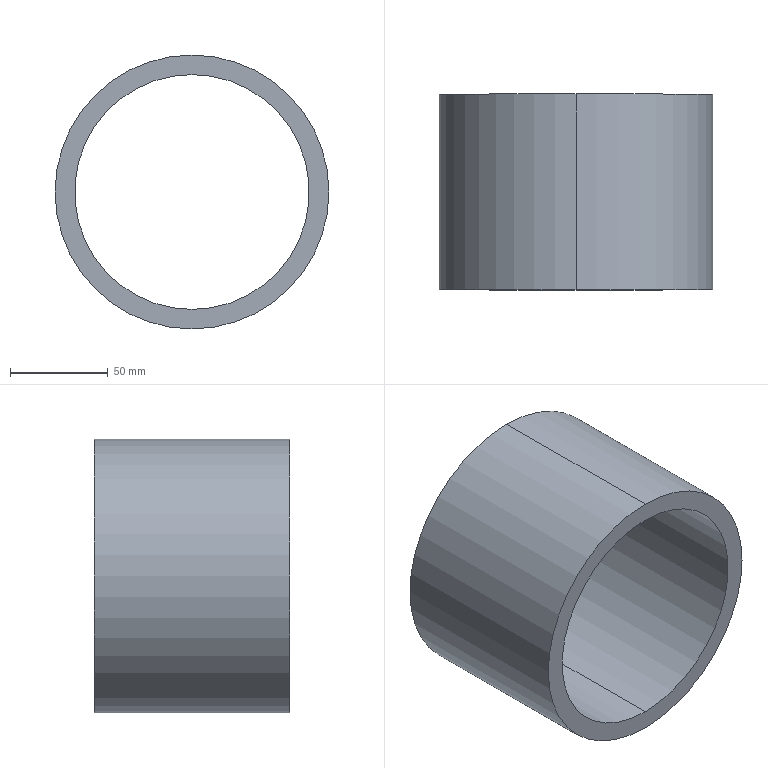Part | SolidWorks | features Extrusion 1 | 1 solid | 6 faces | box 140 x 100 x 140 mm | volume 408407 mm3 | cylinder 4 | plane 2 | commonest cylinder face diameters 120 x2 140 x2
STEP:
#1=CARTESIAN_POINT('',(0.,100.,-60.));
#2=VERTEX_POINT('',#1);
#3=CARTESIAN_POINT('',(0.,100.,60.));
#4=VERTEX_POINT('',#3);
#5=CARTESIAN_POINT('',(0.,100.,0.));
#6=DIRECTION('',(0.,1.,0.));
#7=DIRECTION('',(0.,0.,1.));
#8=AXIS2_PLACEMENT_3D('',#5,#6,#7);
#9=CIRCLE('',#8,60.);
#10=EDGE_CURVE('',#2,#4,#9,.T.);
#11=ORIENTED_EDGE('',*,*,#10,.T.);
#12=CARTESIAN_POINT('',(0.,0.,60.));
#13=VERTEX_POINT('',#12);
#14=CARTESIAN_POINT('',(0.,100.,60.));
#15=DIRECTION('',(0.,-1.,0.));
#16=VECTOR('',#15,1000.);
#17=LINE('',#14,#16);
#18=EDGE_CURVE('',#4,#13,#17,.T.);
#19=ORIENTED_EDGE('',*,*,#18,.T.);
#20=CARTESIAN_POINT('',(0.,0.,-60.));
#21=VERTEX_POINT('',#20);
#22=CARTESIAN_POINT('',(0.,0.,0.));
#23=DIRECTION('',(0.,1.,0.));
#24=DIRECTION('',(0.,0.,1.));
#25=AXIS2_PLACEMENT_3D('',#22,#23,#24);
#26=CIRCLE('',#25,60.);
#27=EDGE_CURVE('',#21,#13,#26,.T.);
#28=ORIENTED_EDGE('',*,*,#27,.F.);
#29=CARTESIAN_POINT('',(0.,100.,-60.));
#30=DIRECTION('',(0.,-1.,0.));
#31=VECTOR('',#30,1000.);
#32=LINE('',#29,#31);
#33=EDGE_CURVE('',#2,#21,#32,.T.);
#34=ORIENTED_EDGE('',*,*,#33,.F.);
#35=EDGE_LOOP('',(#11,#19,#28,#34));
#36=FACE_OUTER_BOUND('',#35,.T.);
#37=CARTESIAN_POINT('',(0.,100.,0.));
#38=DIRECTION('',(0.,-1.,0.));
#39=DIRECTION('',(0.,0.,-1.));
#40=AXIS2_PLACEMENT_3D('',#37,#38,#39);
#41=CYLINDRICAL_SURFACE('',#40,60.);
#42=ADVANCED_FACE('',(#36),#41,.F.);
#43=CARTESIAN_POINT('',(0.,100.,70.));
#44=VERTEX_POINT('',#43);
#45=CARTESIAN_POINT('',(0.,100.,-70.));
#46=VERTEX_POINT('',#45);
#47=CARTESIAN_POINT('',(0.,100.,0.));
#48=DIRECTION('',(0.,1.,0.));
#49=DIRECTION('',(0.,0.,1.));
#50=AXIS2_PLACEMENT_3D('',#47,#48,#49);
#51=CIRCLE('',#50,70.);
#52=EDGE_CURVE('',#44,#46,#51,.T.);
#53=ORIENTED_EDGE('',*,*,#52,.F.);
#54=CARTESIAN_POINT('',(0.,0.,70.));
#55=VERTEX_POINT('',#54);
#56=CARTESIAN_POINT('',(0.,100.,70.));
#57=DIRECTION('',(0.,-1.,0.));
#58=VECTOR('',#57,1000.);
#59=LINE('',#56,#58);
#60=EDGE_CURVE('',#44,#55,#59,.T.);
#61=ORIENTED_EDGE('',*,*,#60,.T.);
#62=CARTESIAN_POINT('',(0.,0.,-70.));
#63=VERTEX_POINT('',#62);
#64=CARTESIAN_POINT('',(0.,0.,0.));
#65=DIRECTION('',(0.,1.,0.));
#66=DIRECTION('',(0.,0.,1.));
#67=AXIS2_PLACEMENT_3D('',#64,#65,#66);
#68=CIRCLE('',#67,70.);
#69=EDGE_CURVE('',#55,#63,#68,.T.);
#70=ORIENTED_EDGE('',*,*,#69,.T.);
#71=CARTESIAN_POINT('',(0.,100.,-70.));
#72=DIRECTION('',(0.,-1.,0.));
#73=VECTOR('',#72,1000.);
#74=LINE('',#71,#73);
#75=EDGE_CURVE('',#46,#63,#74,.T.);
#76=ORIENTED_EDGE('',*,*,#75,.F.);
#77=EDGE_LOOP('',(#53,#61,#70,#76));
#78=FACE_OUTER_BOUND('',#77,.T.);
#79=CARTESIAN_POINT('',(0.,100.,0.));
#80=DIRECTION('',(0.,-1.,0.));
#81=DIRECTION('',(0.,0.,-1.));
#82=AXIS2_PLACEMENT_3D('',#79,#80,#81);
#83=CYLINDRICAL_SURFACE('',#82,70.);
#84=ADVANCED_FACE('',(#78),#83,.T.);
#85=CARTESIAN_POINT('',(0.,100.,0.));
#86=DIRECTION('',(0.,1.,0.));
#87=DIRECTION('',(0.,0.,1.));
#88=AXIS2_PLACEMENT_3D('',#85,#86,#87);
#89=CIRCLE('',#88,70.);
#90=EDGE_CURVE('',#46,#44,#89,.T.);
#91=ORIENTED_EDGE('',*,*,#90,.T.);
#92=ORIENTED_EDGE('',*,*,#52,.T.);
#93=EDGE_LOOP('',(#91,#92));
#94=FACE_OUTER_BOUND('',#93,.T.);
#95=ORIENTED_EDGE('',*,*,#10,.F.);
#96=CARTESIAN_POINT('',(0.,100.,0.));
#97=DIRECTION('',(0.,1.,0.));
#98=DIRECTION('',(0.,0.,1.));
#99=AXIS2_PLACEMENT_3D('',#96,#97,#98);
#100=CIRCLE('',#99,60.);
#101=EDGE_CURVE('',#4,#2,#100,.T.);
#102=ORIENTED_EDGE('',*,*,#101,.F.);
#103=EDGE_LOOP('',(#95,#102));
#104=FACE_BOUND('',#103,.T.);
#105=CARTESIAN_POINT('',(0.,100.,0.));
#106=DIRECTION('',(0.,1.,0.));
#107=DIRECTION('',(0.,0.,1.));
#108=AXIS2_PLACEMENT_3D('',#105,#106,#107);
#109=PLANE('',#108);
#110=ADVANCED_FACE('',(#94,#104),#109,.T.);
#111=CARTESIAN_POINT('',(0.,0.,0.));
#112=DIRECTION('',(0.,1.,0.));
#113=DIRECTION('',(0.,0.,1.));
#114=AXIS2_PLACEMENT_3D('',#111,#112,#113);
#115=CIRCLE('',#114,70.);
#116=EDGE_CURVE('',#63,#55,#115,.T.);
#117=ORIENTED_EDGE('',*,*,#116,.F.);
#118=ORIENTED_EDGE('',*,*,#69,.F.);
#119=EDGE_LOOP('',(#117,#118));
#120=FACE_OUTER_BOUND('',#119,.T.);
#121=ORIENTED_EDGE('',*,*,#27,.T.);
#122=CARTESIAN_POINT('',(0.,0.,0.));
#123=DIRECTION('',(0.,1.,0.));
#124=DIRECTION('',(0.,0.,1.));
#125=AXIS2_PLACEMENT_3D('',#122,#123,#124);
#126=CIRCLE('',#125,60.);
#127=EDGE_CURVE('',#13,#21,#126,.T.);
#128=ORIENTED_EDGE('',*,*,#127,.T.);
#129=EDGE_LOOP('',(#121,#128));
#130=FACE_BOUND('',#129,.T.);
#131=CARTESIAN_POINT('',(0.,0.,0.));
#132=DIRECTION('',(0.,1.,0.));
#133=DIRECTION('',(0.,0.,1.));
#134=AXIS2_PLACEMENT_3D('',#131,#132,#133);
#135=PLANE('',#134);
#136=ADVANCED_FACE('',(#120,#130),#135,.F.);
#137=ORIENTED_EDGE('',*,*,#60,.F.);
#138=ORIENTED_EDGE('',*,*,#90,.F.);
#139=ORIENTED_EDGE('',*,*,#75,.T.);
#140=ORIENTED_EDGE('',*,*,#116,.T.);
#141=EDGE_LOOP('',(#137,#138,#139,#140));
#142=FACE_OUTER_BOUND('',#141,.T.);
#143=CARTESIAN_POINT('',(0.,100.,0.));
#144=DIRECTION('',(0.,-1.,0.));
#145=DIRECTION('',(0.,0.,-1.));
#146=AXIS2_PLACEMENT_3D('',#143,#144,#145);
#147=CYLINDRICAL_SURFACE('',#146,70.);
#148=ADVANCED_FACE('',(#142),#147,.T.);
#149=ORIENTED_EDGE('',*,*,#18,.F.);
#150=ORIENTED_EDGE('',*,*,#101,.T.);
#151=ORIENTED_EDGE('',*,*,#33,.T.);
#152=ORIENTED_EDGE('',*,*,#127,.F.);
#153=EDGE_LOOP('',(#149,#150,#151,#152));
#154=FACE_OUTER_BOUND('',#153,.T.);
#155=CARTESIAN_POINT('',(0.,100.,0.));
#156=DIRECTION('',(0.,-1.,0.));
#157=DIRECTION('',(0.,0.,-1.));
#158=AXIS2_PLACEMENT_3D('',#155,#156,#157);
#159=CYLINDRICAL_SURFACE('',#158,60.);
#160=ADVANCED_FACE('',(#154),#159,.F.);
#161=CLOSED_SHELL('',(#42,#84,#110,#136,#148,#160));
#162=MANIFOLD_SOLID_BREP('',#161);
#163=CARTESIAN_POINT('',(0.,0.,0.));
#164=DIRECTION('',(0.,0.,1.));
#165=DIRECTION('',(1.,0.,0.));
#166=AXIS2_PLACEMENT_3D('',#163,#164,#165);
#167=(LENGTH_UNIT()NAMED_UNIT(*)SI_UNIT(.MILLI.,.METRE.));
#168=UNCERTAINTY_MEASURE_WITH_UNIT(LENGTH_MEASURE(0.00001),#167,'','');
#169=(NAMED_UNIT(*)PLANE_ANGLE_UNIT()SI_UNIT($,.RADIAN.));
#170=(NAMED_UNIT(*)SI_UNIT($,.STERADIAN.)SOLID_ANGLE_UNIT());
#171=(GEOMETRIC_REPRESENTATION_CONTEXT(3)GLOBAL_UNCERTAINTY_ASSIGNED_CONTEXT((#168))GLOBAL_UNIT_ASSIGNED_CONTEXT((#167,#169,#170))REPRESENTATION_CONTEXT('',''));
#172=ADVANCED_BREP_SHAPE_REPRESENTATION('',(#162,#166),#171);